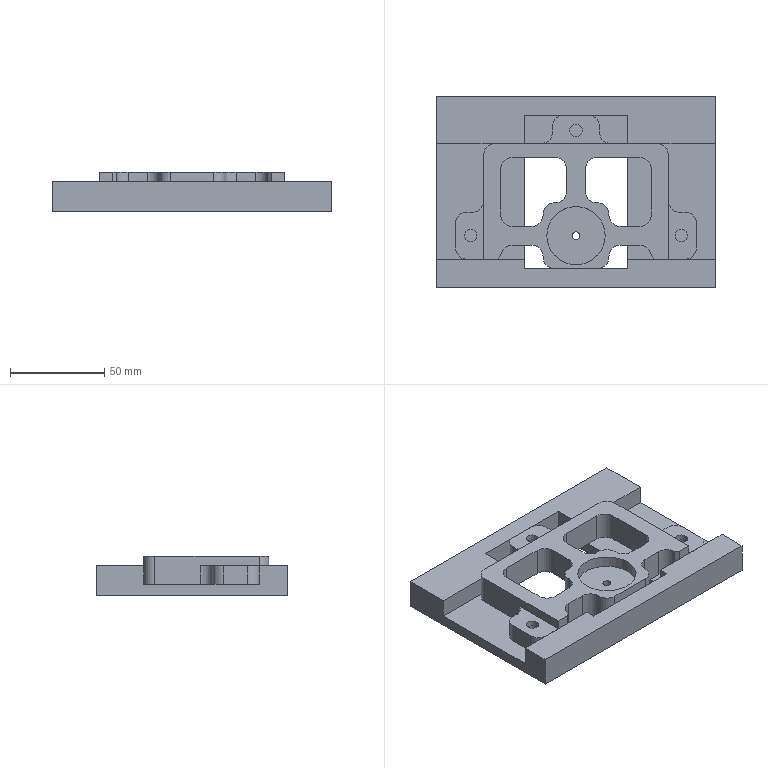NC program | NX | posted with a generic post | part box 148 x 101.5 x 21 mm
Whole program, first 1776 of 1973 lines:
N10 G17 G21 G94 G90
(FLOOR_WALL_COPY_1 , TOOL : D10)
N12 T04 M6
N14 G54
N16 G17 G0 G90 X72. Y-40.747 S9505 M3
N18 G43 Z30. H4
N20 Z6.025
N22 G94 G1 Z3.025 F2500.
N24 X69.
N26 X-69.
N28 Y-35.903
N30 X69.
N32 Y-31.06
N34 X-69.
N36 Y-26.216
N38 X69.
N40 Y-21.373
N42 X-69.
N44 Y-16.529
N46 X69.
N48 Y-11.686
N50 X-69.
N52 Y-6.842
N54 X69.
N56 Y-1.999
N58 X-69.
N60 Y2.845
N62 X69.
N64 Y7.689
N66 X-69.
N68 Y12.532
N70 X69.
N72 Y17.376
N74 X-69.
N76 Y22.219
N78 X69.
N80 Y27.063
N82 X-69.
N84 Y31.906
N86 X69.
N88 Y36.75
N90 X-69.
N92 X-72.
N94 Z6.025
N96 G0 Z30.
N98 X72. Y-40.747
N100 Z5.05
N102 G1 Z2.05
N104 X69.
N106 X-69.
N108 Y-35.903
N110 X69.
N112 Y-31.06
N114 X-69.
N116 Y-26.216
N118 X69.
N120 Y-21.373
N122 X-69.
N124 Y-16.529
N126 X69.
N128 Y-11.686
N130 X-69.
N132 Y-6.842
N134 X69.
N136 Y-1.999
N138 X-69.
N140 Y2.845
N142 X69.
N144 Y7.689
N146 X-69.
N148 Y12.532
N150 X69.
N152 Y17.376
N154 X-69.
N156 Y22.219
N158 X69.
N160 Y27.063
N162 X-69.
N164 Y31.906
N166 X69.
N168 Y36.75
N170 X-69.
N172 X-72.
N174 Z5.05
N176 G0 Z30.
N178 X72. Y-40.747
N180 Z4.075
N182 G1 Z1.075
N184 X69.
N186 X-69.
N188 Y-35.903
N190 X69.
N192 Y-31.06
N194 X-69.
N196 Y-26.216
N198 X69.
N200 Y-21.373
N202 X-69.
N204 Y-16.529
N206 X69.
N208 Y-11.686
N210 X-69.
N212 Y-6.842
N214 X69.
N216 Y-1.999
N218 X-69.
N220 Y2.845
N222 X69.
N224 Y7.689
N226 X-69.
N228 Y12.532
N230 X69.
N232 Y17.376
N234 X-69.
N236 Y22.219
N238 X69.
N240 Y27.063
N242 X-69.
N244 Y31.906
N246 X69.
N248 Y36.75
N250 X-69.
N252 X-72.
N254 Z4.075
N256 G0 Z30.
N258 X72. Y-40.747
N260 Z3.1
N262 G1 Z0.1
N264 X69.
N266 X-69.
N268 Y-35.903
N270 X69.
N272 Y-31.06
N274 X-69.
N276 Y-26.216
N278 X69.
N280 Y-21.373
N282 X-69.
N284 Y-16.529
N286 X69.
N288 Y-11.686
N290 X-69.
N292 Y-6.842
N294 X69.
N296 Y-1.999
N298 X-69.
N300 Y2.845
N302 X69.
N304 Y7.689
N306 X-69.
N308 Y12.532
N310 X69.
N312 Y17.376
N314 X-69.
N316 Y22.219
N318 X69.
N320 Y27.063
N322 X-69.
N324 Y31.906
N326 X69.
N328 Y36.75
N330 X-69.
N332 X-72.
N334 Z3.1
N336 G0 Z30.
(FLOOR_WALL_COPY_1_COPY , TOOL : D10)
N338 X21.949 Y-33.897
N340 Z3.021
N342 G1 Z0.021 F2200.
N344 X17.776 Y-31.299
N346 G3 X17.647 Y-31.75 R0.853
N348 G1 Y-34.75
N350 G2 X6.5 Y-45.897 R11.147
N352 G1 X-6.5
N354 G2 X-17.647 Y-34.75 R11.147
N356 G1 Y-31.75
N358 G3 X-18.5 Y-30.897 R0.853
N360 G1 X-43.
N362 G2 X-54.147 Y-19.75 R11.147
N364 G1 Y4.75
N366 G3 X-55. Y5.603 R0.853
N368 G1 X-58.
N370 G2 X-69.147 Y16.75 R11.147
N372 G1 Y29.75
N374 G2 X-58. Y40.897 R11.147
N376 G1 X-39.946
N378 X-34.979 Y36.231
N380 X-34.851 Y34.197
N382 G3 X-34. Y33.397 R0.853
N384 G1 X-23.5
N386 G3 X-22.679 Y34.019 R0.853
N388 G1 X-22.65 Y34.011
N390 Y11.75
N392 G3 X-11.5 Y0.6 R11.15
N394 G1 X11.5
N396 G3 X22.65 Y11.75 R11.15
N398 G1 Y34.011
N400 X22.679 Y34.019
N402 G3 X23.5 Y33.397 R0.853
N404 G1 X34.
N406 G3 X34.855 Y34.255 R0.855
N408 G1 X34.979 Y36.231
N410 X39.946 Y40.897
N412 X58.
N414 G2 X69.147 Y29.75 R11.147
N416 G1 Y16.75
N418 G2 X58. Y5.603 R11.147
N420 G1 X55.
N422 G3 X54.147 Y4.75 R0.853
N424 G1 Y-19.75
N426 G2 X43. Y-30.897 R11.147
N428 G1 X18.5
N430 G3 X17.776 Y-31.299 R0.853
N432 G1 X13.531 Y-28.657
N434 G3 X12.647 Y-31.75 R5.853
N436 G1 Y-34.75
N438 G2 X6.5 Y-40.897 R6.147
N440 G1 X-6.5
N442 G2 X-12.647 Y-34.75 R6.147
N444 G1 Y-31.75
N446 G3 X-18.5 Y-25.897 R5.853
N448 G1 X-43.
N450 G2 X-49.147 Y-19.75 R6.147
N452 G1 Y4.75
N454 G3 X-55. Y10.603 R5.853
N456 G1 X-58.
N458 G2 X-64.147 Y16.75 R6.147
N460 G1 Y29.75
N462 G2 X-58. Y35.897 R6.147
N464 G1 X-41.926
N466 X-39.845 Y33.942
N468 G3 X-34. Y28.397 R5.853
N470 G1 X-27.65
N472 Y11.75
N474 G3 X-11.5 Y-4.4 R16.15
N476 G1 X11.5
N478 G3 X27.65 Y11.75 R16.15
N480 G1 Y28.397
N482 X34.002
N484 G3 X39.567 Y32.442 R5.853
N486 X39.845 Y33.942 R5.853
N488 G1 X41.926 Y35.897
N490 X58.
N492 G2 X64.147 Y29.75 R6.147
N494 G1 Y16.75
N496 G2 X58. Y10.603 R6.147
N498 G1 X55.
N500 G3 X49.147 Y4.75 R5.853
N502 G1 Y-19.75
N504 G2 X43. Y-25.897 R6.147
N506 G1 X18.5
N508 G3 X13.531 Y-28.657 R5.853
N510 G1 X9.286 Y-26.015
N512 G3 X7.647 Y-31.75 R10.853
N514 G1 Y-34.75
N516 G2 X6.5 Y-35.897 R1.147
N518 G1 X-6.5
N520 G2 X-7.647 Y-34.75 R1.147
N522 G1 Y-31.75
N524 G3 X-18.5 Y-20.897 R10.853
N526 G1 X-43.
N528 G2 X-44.147 Y-19.75 R1.147
N530 G1 Y4.75
N532 G3 X-55. Y15.603 R10.853
N534 G1 X-58.
N536 G2 X-59.147 Y16.75 R1.147
N538 G1 Y29.75
N540 G2 X-58. Y30.897 R1.147
N542 G1 X-44.322
N544 G3 X-34. Y23.397 R10.853
N546 G1 X-32.65
N548 Y11.75
N550 G3 X-11.5 Y-9.4 R21.15
N552 G1 X11.5
N554 G3 X32.65 Y11.75 R21.15
N556 G1 Y23.397
N558 X34.004
N560 G3 X44.322 Y30.897 R10.853
N562 G1 X58.
N564 G2 X59.147 Y29.75 R1.147
N566 G1 Y16.75
N568 G2 X58. Y15.603 R1.147
N570 G1 X55.
N572 G3 X44.147 Y4.75 R10.853
N574 G1 Y-19.75
N576 G2 X43. Y-20.897 R1.147
N578 G1 X18.5
N580 G3 X9.286 Y-26.015 R10.853
N582 G1 X5.041 Y-23.373
N584 G3 X2.67 Y-30.897 R15.853
N586 G1 X-2.67
N588 G3 X-18.5 Y-15.897 R15.853
N590 G1 X-39.147
N592 Y4.75
N594 G3 X-54.147 Y20.58 R15.853
N596 G1 Y25.897
N598 X-47.474
N600 G3 X-37.65 Y18.823 R15.853
N602 G1 Y11.75
N604 G3 X-29.455 Y-7.262 R26.15
N606 G1 X-32.888 Y-10.897
N608 X-34.147
N610 Y-9.638
N612 G3 X-32.888 Y-10.897 R31.15
N614 G1 X-29.455 Y-7.262
N616 G3 X-11.5 Y-14.4 R26.15
N618 G1 X11.5
N620 G3 X37.65 Y11.75 R26.15
N622 G1 Y18.823
N624 G3 X47.474 Y25.897 R15.853
N626 G1 X54.147
N628 Y20.58
N630 G3 X39.147 Y4.75 R15.853
N632 G1 Y-15.897
N634 X32.888
N636 Y-10.897
N638 G3 X34.147 Y-9.638 R31.15
N640 G1 Y-10.897
N642 X32.888
N644 Y-15.897
N646 X18.5
N648 G3 X5.041 Y-23.373 R15.853
N650 G1 X0.796 Y-20.731
N652 G3 X0. Y-22.127 R20.853
N654 X-1.697 Y-19.4 R20.853
N656 G1 X1.697
N658 G3 X0.796 Y-20.731 R20.853
N660 G1 X3.343 Y-22.316
N662 Z3.021
N664 G0 Z30.
N666 X21.949 Y-33.897
N668 Z2.043
N670 G1 Z-0.957
N672 X17.776 Y-31.299
N674 G3 X17.647 Y-31.75 R0.853
N676 G1 Y-34.75
N678 G2 X6.5 Y-45.897 R11.147
N680 G1 X-6.5
N682 G2 X-17.647 Y-34.75 R11.147
N684 G1 Y-31.75
N686 G3 X-18.5 Y-30.897 R0.853
N688 G1 X-43.
N690 G2 X-54.147 Y-19.75 R11.147
N692 G1 Y4.75
N694 G3 X-55. Y5.603 R0.853
N696 G1 X-58.
N698 G2 X-69.147 Y16.75 R11.147
N700 G1 Y29.75
N702 G2 X-58. Y40.897 R11.147
N704 G1 X-39.946
N706 X-34.979 Y36.231
N708 X-34.851 Y34.197
N710 G3 X-34. Y33.397 R0.853
N712 G1 X-23.5
N714 G3 X-22.679 Y34.019 R0.853
N716 G1 X-22.65 Y34.011
N718 Y11.75
N720 G3 X-11.5 Y0.6 R11.15
N722 G1 X11.5
N724 G3 X22.65 Y11.75 R11.15
N726 G1 Y34.011
N728 X22.679 Y34.019
N730 G3 X23.5 Y33.397 R0.853
N732 G1 X34.
N734 G3 X34.855 Y34.255 R0.855
N736 G1 X34.979 Y36.231
N738 X39.946 Y40.897
N740 X58.
N742 G2 X69.147 Y29.75 R11.147
N744 G1 Y16.75
N746 G2 X58. Y5.603 R11.147
N748 G1 X55.
N750 G3 X54.147 Y4.75 R0.853
N752 G1 Y-19.75
N754 G2 X43. Y-30.897 R11.147
N756 G1 X18.5
N758 G3 X17.776 Y-31.299 R0.853
N760 G1 X13.531 Y-28.657
N762 G3 X12.647 Y-31.75 R5.853
N764 G1 Y-34.75
N766 G2 X6.5 Y-40.897 R6.147
N768 G1 X-6.5
N770 G2 X-12.647 Y-34.75 R6.147
N772 G1 Y-31.75
N774 G3 X-18.5 Y-25.897 R5.853
N776 G1 X-43.
N778 G2 X-49.147 Y-19.75 R6.147
N780 G1 Y4.75
N782 G3 X-55. Y10.603 R5.853
N784 G1 X-58.
N786 G2 X-64.147 Y16.75 R6.147
N788 G1 Y29.75
N790 G2 X-58. Y35.897 R6.147
N792 G1 X-41.926
N794 X-39.845 Y33.942
N796 G3 X-34. Y28.397 R5.853
N798 G1 X-27.65
N800 Y11.75
N802 G3 X-11.5 Y-4.4 R16.15
N804 G1 X11.5
N806 G3 X27.65 Y11.75 R16.15
N808 G1 Y28.397
N810 X34.002
N812 G3 X39.567 Y32.442 R5.853
N814 X39.845 Y33.942 R5.853
N816 G1 X41.926 Y35.897
N818 X58.
N820 G2 X64.147 Y29.75 R6.147
N822 G1 Y16.75
N824 G2 X58. Y10.603 R6.147
N826 G1 X55.
N828 G3 X49.147 Y4.75 R5.853
N830 G1 Y-19.75
N832 G2 X43. Y-25.897 R6.147
N834 G1 X18.5
N836 G3 X13.531 Y-28.657 R5.853
N838 G1 X9.286 Y-26.015
N840 G3 X7.647 Y-31.75 R10.853
N842 G1 Y-34.75
N844 G2 X6.5 Y-35.897 R1.147
N846 G1 X-6.5
N848 G2 X-7.647 Y-34.75 R1.147
N850 G1 Y-31.75
N852 G3 X-18.5 Y-20.897 R10.853
N854 G1 X-43.
N856 G2 X-44.147 Y-19.75 R1.147
N858 G1 Y4.75
N860 G3 X-55. Y15.603 R10.853
N862 G1 X-58.
N864 G2 X-59.147 Y16.75 R1.147
N866 G1 Y29.75
N868 G2 X-58. Y30.897 R1.147
N870 G1 X-44.322
N872 G3 X-34. Y23.397 R10.853
N874 G1 X-32.65
N876 Y11.75
N878 G3 X-11.5 Y-9.4 R21.15
N880 G1 X11.5
N882 G3 X32.65 Y11.75 R21.15
N884 G1 Y23.397
N886 X34.004
N888 G3 X44.322 Y30.897 R10.853
N890 G1 X58.
N892 G2 X59.147 Y29.75 R1.147
N894 G1 Y16.75
N896 G2 X58. Y15.603 R1.147
N898 G1 X55.
N900 G3 X44.147 Y4.75 R10.853
N902 G1 Y-19.75
N904 G2 X43. Y-20.897 R1.147
N906 G1 X18.5
N908 G3 X9.286 Y-26.015 R10.853
N910 G1 X5.041 Y-23.373
N912 G3 X2.67 Y-30.897 R15.853
N914 G1 X-2.67
N916 G3 X-18.5 Y-15.897 R15.853
N918 G1 X-39.147
N920 Y4.75
N922 G3 X-54.147 Y20.58 R15.853
N924 G1 Y25.897
N926 X-47.474
N928 G3 X-37.65 Y18.823 R15.853
N930 G1 Y11.75
N932 G3 X-29.455 Y-7.262 R26.15
N934 G1 X-32.888 Y-10.897
N936 X-34.147
N938 Y-9.638
N940 G3 X-32.888 Y-10.897 R31.15
N942 G1 X-29.455 Y-7.262
N944 G3 X-11.5 Y-14.4 R26.15
N946 G1 X11.5
N948 G3 X37.65 Y11.75 R26.15
N950 G1 Y18.823
N952 G3 X47.474 Y25.897 R15.853
N954 G1 X54.147
N956 Y20.58
N958 G3 X39.147 Y4.75 R15.853
N960 G1 Y-15.897
N962 X32.888
N964 Y-10.897
N966 G3 X34.147 Y-9.638 R31.15
N968 G1 Y-10.897
N970 X32.888
N972 Y-15.897
N974 X18.5
N976 G3 X5.041 Y-23.373 R15.853
N978 G1 X0.796 Y-20.731
N980 G3 X0. Y-22.127 R20.853
N982 X-1.697 Y-19.4 R20.853
N984 G1 X1.697
N986 G3 X0.796 Y-20.731 R20.853
N988 G1 X3.343 Y-22.316
N990 Z2.043
N992 G0 Z30.
N994 X21.949 Y-33.897
N996 Z1.064
N998 G1 Z-1.936
N1000 X17.776 Y-31.299
N1002 G3 X17.647 Y-31.75 R0.853
N1004 G1 Y-34.75
N1006 G2 X6.5 Y-45.897 R11.147
N1008 G1 X-6.5
N1010 G2 X-17.647 Y-34.75 R11.147
N1012 G1 Y-31.75
N1014 G3 X-18.5 Y-30.897 R0.853
N1016 G1 X-43.
N1018 G2 X-54.147 Y-19.75 R11.147
N1020 G1 Y4.75
N1022 G3 X-55. Y5.603 R0.853
N1024 G1 X-58.
N1026 G2 X-69.147 Y16.75 R11.147
N1028 G1 Y29.75
N1030 G2 X-58. Y40.897 R11.147
N1032 G1 X-39.946
N1034 X-34.979 Y36.231
N1036 X-34.851 Y34.197
N1038 G3 X-34. Y33.397 R0.853
N1040 G1 X-23.5
N1042 G3 X-22.679 Y34.019 R0.853
N1044 G1 X-22.65 Y34.011
N1046 Y11.75
N1048 G3 X-11.5 Y0.6 R11.15
N1050 G1 X11.5
N1052 G3 X22.65 Y11.75 R11.15
N1054 G1 Y34.011
N1056 X22.679 Y34.019
N1058 G3 X23.5 Y33.397 R0.853
N1060 G1 X34.
N1062 G3 X34.855 Y34.255 R0.855
N1064 G1 X34.979 Y36.231
N1066 X39.946 Y40.897
N1068 X58.
N1070 G2 X69.147 Y29.75 R11.147
N1072 G1 Y16.75
N1074 G2 X58. Y5.603 R11.147
N1076 G1 X55.
N1078 G3 X54.147 Y4.75 R0.853
N1080 G1 Y-19.75
N1082 G2 X43. Y-30.897 R11.147
N1084 G1 X18.5
N1086 G3 X17.776 Y-31.299 R0.853
N1088 G1 X13.531 Y-28.657
N1090 G3 X12.647 Y-31.75 R5.853
N1092 G1 Y-34.75
N1094 G2 X6.5 Y-40.897 R6.147
N1096 G1 X-6.5
N1098 G2 X-12.647 Y-34.75 R6.147
N1100 G1 Y-31.75
N1102 G3 X-18.5 Y-25.897 R5.853
N1104 G1 X-43.
N1106 G2 X-49.147 Y-19.75 R6.147
N1108 G1 Y4.75
N1110 G3 X-55. Y10.603 R5.853
N1112 G1 X-58.
N1114 G2 X-64.147 Y16.75 R6.147
N1116 G1 Y29.75
N1118 G2 X-58. Y35.897 R6.147
N1120 G1 X-41.926
N1122 X-39.845 Y33.942
N1124 G3 X-34. Y28.397 R5.853
N1126 G1 X-27.65
N1128 Y11.75
N1130 G3 X-11.5 Y-4.4 R16.15
N1132 G1 X11.5
N1134 G3 X27.65 Y11.75 R16.15
N1136 G1 Y28.397
N1138 X34.002
N1140 G3 X39.567 Y32.442 R5.853
N1142 X39.845 Y33.942 R5.853
N1144 G1 X41.926 Y35.897
N1146 X58.
N1148 G2 X64.147 Y29.75 R6.147
N1150 G1 Y16.75
N1152 G2 X58. Y10.603 R6.147
N1154 G1 X55.
N1156 G3 X49.147 Y4.75 R5.853
N1158 G1 Y-19.75
N1160 G2 X43. Y-25.897 R6.147
N1162 G1 X18.5
N1164 G3 X13.531 Y-28.657 R5.853
N1166 G1 X9.286 Y-26.015
N1168 G3 X7.647 Y-31.75 R10.853
N1170 G1 Y-34.75
N1172 G2 X6.5 Y-35.897 R1.147
N1174 G1 X-6.5
N1176 G2 X-7.647 Y-34.75 R1.147
N1178 G1 Y-31.75
N1180 G3 X-18.5 Y-20.897 R10.853
N1182 G1 X-43.
N1184 G2 X-44.147 Y-19.75 R1.147
N1186 G1 Y4.75
N1188 G3 X-55. Y15.603 R10.853
N1190 G1 X-58.
N1192 G2 X-59.147 Y16.75 R1.147
N1194 G1 Y29.75
N1196 G2 X-58. Y30.897 R1.147
N1198 G1 X-44.322
N1200 G3 X-34. Y23.397 R10.853
N1202 G1 X-32.65
N1204 Y11.75
N1206 G3 X-11.5 Y-9.4 R21.15
N1208 G1 X11.5
N1210 G3 X32.65 Y11.75 R21.15
N1212 G1 Y23.397
N1214 X34.004
N1216 G3 X44.322 Y30.897 R10.853
N1218 G1 X58.
N1220 G2 X59.147 Y29.75 R1.147
N1222 G1 Y16.75
N1224 G2 X58. Y15.603 R1.147
N1226 G1 X55.
N1228 G3 X44.147 Y4.75 R10.853
N1230 G1 Y-19.75
N1232 G2 X43. Y-20.897 R1.147
N1234 G1 X18.5
N1236 G3 X9.286 Y-26.015 R10.853
N1238 G1 X5.041 Y-23.373
N1240 G3 X2.67 Y-30.897 R15.853
N1242 G1 X-2.67
N1244 G3 X-18.5 Y-15.897 R15.853
N1246 G1 X-39.147
N1248 Y4.75
N1250 G3 X-54.147 Y20.58 R15.853
N1252 G1 Y25.897
N1254 X-47.474
N1256 G3 X-37.65 Y18.823 R15.853
N1258 G1 Y11.75
N1260 G3 X-29.455 Y-7.262 R26.15
N1262 G1 X-32.888 Y-10.897
N1264 X-34.147
N1266 Y-9.638
N1268 G3 X-32.888 Y-10.897 R31.15
N1270 G1 X-29.455 Y-7.262
N1272 G3 X-11.5 Y-14.4 R26.15
N1274 G1 X11.5
N1276 G3 X37.65 Y11.75 R26.15
N1278 G1 Y18.823
N1280 G3 X47.474 Y25.897 R15.853
N1282 G1 X54.147
N1284 Y20.58
N1286 G3 X39.147 Y4.75 R15.853
N1288 G1 Y-15.897
N1290 X32.888
N1292 Y-10.897
N1294 G3 X34.147 Y-9.638 R31.15
N1296 G1 Y-10.897
N1298 X32.888
N1300 Y-15.897
N1302 X18.5
N1304 G3 X5.041 Y-23.373 R15.853
N1306 G1 X0.796 Y-20.731
N1308 G3 X0. Y-22.127 R20.853
N1310 X-1.697 Y-19.4 R20.853
N1312 G1 X1.697
N1314 G3 X0.796 Y-20.731 R20.853
N1316 G1 X3.343 Y-22.316
N1318 Z1.064
N1320 G0 Z30.
N1322 X21.949 Y-33.897
N1324 Z0.086
N1326 G1 Z-2.914
N1328 X17.776 Y-31.299
N1330 G3 X17.647 Y-31.75 R0.853
N1332 G1 Y-34.75
N1334 G2 X6.5 Y-45.897 R11.147
N1336 G1 X-6.5
N1338 G2 X-17.647 Y-34.75 R11.147
N1340 G1 Y-31.75
N1342 G3 X-18.5 Y-30.897 R0.853
N1344 G1 X-43.
N1346 G2 X-54.147 Y-19.75 R11.147
N1348 G1 Y4.75
N1350 G3 X-55. Y5.603 R0.853
N1352 G1 X-58.
N1354 G2 X-69.147 Y16.75 R11.147
N1356 G1 Y29.75
N1358 G2 X-58. Y40.897 R11.147
N1360 G1 X-39.946
N1362 X-34.979 Y36.231
N1364 X-34.851 Y34.197
N1366 G3 X-34. Y33.397 R0.853
N1368 G1 X-23.5
N1370 G3 X-22.679 Y34.019 R0.853
N1372 G1 X-22.65 Y34.011
N1374 Y11.75
N1376 G3 X-11.5 Y0.6 R11.15
N1378 G1 X11.5
N1380 G3 X22.65 Y11.75 R11.15
N1382 G1 Y34.011
N1384 X22.679 Y34.019
N1386 G3 X23.5 Y33.397 R0.853
N1388 G1 X34.
N1390 G3 X34.855 Y34.255 R0.855
N1392 G1 X34.979 Y36.231
N1394 X39.946 Y40.897
N1396 X58.
N1398 G2 X69.147 Y29.75 R11.147
N1400 G1 Y16.75
N1402 G2 X58. Y5.603 R11.147
N1404 G1 X55.
N1406 G3 X54.147 Y4.75 R0.853
N1408 G1 Y-19.75
N1410 G2 X43. Y-30.897 R11.147
N1412 G1 X18.5
N1414 G3 X17.776 Y-31.299 R0.853
N1416 G1 X13.531 Y-28.657
N1418 G3 X12.647 Y-31.75 R5.853
N1420 G1 Y-34.75
N1422 G2 X6.5 Y-40.897 R6.147
N1424 G1 X-6.5
N1426 G2 X-12.647 Y-34.75 R6.147
N1428 G1 Y-31.75
N1430 G3 X-18.5 Y-25.897 R5.853
N1432 G1 X-43.
N1434 G2 X-49.147 Y-19.75 R6.147
N1436 G1 Y4.75
N1438 G3 X-55. Y10.603 R5.853
N1440 G1 X-58.
N1442 G2 X-64.147 Y16.75 R6.147
N1444 G1 Y29.75
N1446 G2 X-58. Y35.897 R6.147
N1448 G1 X-41.926
N1450 X-39.845 Y33.942
N1452 G3 X-34. Y28.397 R5.853
N1454 G1 X-27.65
N1456 Y11.75
N1458 G3 X-11.5 Y-4.4 R16.15
N1460 G1 X11.5
N1462 G3 X27.65 Y11.75 R16.15
N1464 G1 Y28.397
N1466 X34.002
N1468 G3 X39.567 Y32.442 R5.853
N1470 X39.845 Y33.942 R5.853
N1472 G1 X41.926 Y35.897
N1474 X58.
N1476 G2 X64.147 Y29.75 R6.147
N1478 G1 Y16.75
N1480 G2 X58. Y10.603 R6.147
N1482 G1 X55.
N1484 G3 X49.147 Y4.75 R5.853
N1486 G1 Y-19.75
N1488 G2 X43. Y-25.897 R6.147
N1490 G1 X18.5
N1492 G3 X13.531 Y-28.657 R5.853
N1494 G1 X9.286 Y-26.015
N1496 G3 X7.647 Y-31.75 R10.853
N1498 G1 Y-34.75
N1500 G2 X6.5 Y-35.897 R1.147
N1502 G1 X-6.5
N1504 G2 X-7.647 Y-34.75 R1.147
N1506 G1 Y-31.75
N1508 G3 X-18.5 Y-20.897 R10.853
N1510 G1 X-43.
N1512 G2 X-44.147 Y-19.75 R1.147
N1514 G1 Y4.75
N1516 G3 X-55. Y15.603 R10.853
N1518 G1 X-58.
N1520 G2 X-59.147 Y16.75 R1.147
N1522 G1 Y29.75
N1524 G2 X-58. Y30.897 R1.147
N1526 G1 X-44.322
N1528 G3 X-34. Y23.397 R10.853
N1530 G1 X-32.65
N1532 Y11.75
N1534 G3 X-11.5 Y-9.4 R21.15
N1536 G1 X11.5
N1538 G3 X32.65 Y11.75 R21.15
N1540 G1 Y23.397
N1542 X34.004
N1544 G3 X44.322 Y30.897 R10.853
N1546 G1 X58.
N1548 G2 X59.147 Y29.75 R1.147
N1550 G1 Y16.75
N1552 G2 X58. Y15.603 R1.147
N1554 G1 X55.
N1556 G3 X44.147 Y4.75 R10.853
N1558 G1 Y-19.75
N1560 G2 X43. Y-20.897 R1.147
N1562 G1 X18.5
N1564 G3 X9.286 Y-26.015 R10.853
N1566 G1 X5.041 Y-23.373
N1568 G3 X2.67 Y-30.897 R15.853
N1570 G1 X-2.67
N1572 G3 X-18.5 Y-15.897 R15.853
N1574 G1 X-39.147
N1576 Y4.75
N1578 G3 X-54.147 Y20.58 R15.853
N1580 G1 Y25.897
N1582 X-47.474
N1584 G3 X-37.65 Y18.823 R15.853
N1586 G1 Y11.75
N1588 G3 X-29.455 Y-7.262 R26.15
N1590 G1 X-32.888 Y-10.897
N1592 X-34.147
N1594 Y-9.638
N1596 G3 X-32.888 Y-10.897 R31.15
N1598 G1 X-29.455 Y-7.262
N1600 G3 X-11.5 Y-14.4 R26.15
N1602 G1 X11.5
N1604 G3 X37.65 Y11.75 R26.15
N1606 G1 Y18.823
N1608 G3 X47.474 Y25.897 R15.853
N1610 G1 X54.147
N1612 Y20.58
N1614 G3 X39.147 Y4.75 R15.853
N1616 G1 Y-15.897
N1618 X32.888
N1620 Y-10.897
N1622 G3 X34.147 Y-9.638 R31.15
N1624 G1 Y-10.897
N1626 X32.888
N1628 Y-15.897
N1630 X18.5
N1632 G3 X5.041 Y-23.373 R15.853
N1634 G1 X0.796 Y-20.731
N1636 G3 X0. Y-22.127 R20.853
N1638 X-1.697 Y-19.4 R20.853
N1640 G1 X1.697
N1642 G3 X0.796 Y-20.731 R20.853
N1644 G1 X3.343 Y-22.316
N1646 Z0.086
N1648 G0 Z30.
N1650 X21.949 Y-33.897
N1652 Z-0.893
N1654 G1 Z-3.893
N1656 X17.776 Y-31.299
N1658 G3 X17.647 Y-31.75 R0.853
N1660 G1 Y-34.75
N1662 G2 X6.5 Y-45.897 R11.147
N1664 G1 X-6.5
N1666 G2 X-17.647 Y-34.75 R11.147
N1668 G1 Y-31.75
N1670 G3 X-18.5 Y-30.897 R0.853
N1672 G1 X-43.
N1674 G2 X-54.147 Y-19.75 R11.147
N1676 G1 Y4.75
N1678 G3 X-55. Y5.603 R0.853
N1680 G1 X-58.
N1682 G2 X-69.147 Y16.75 R11.147
N1684 G1 Y29.75
N1686 G2 X-58. Y40.897 R11.147
N1688 G1 X-39.946
N1690 X-34.979 Y36.231
N1692 X-34.851 Y34.197
N1694 G3 X-34. Y33.397 R0.853
N1696 G1 X-23.5
N1698 G3 X-22.679 Y34.019 R0.853
N1700 G1 X-22.65 Y34.011
N1702 Y11.75
N1704 G3 X-11.5 Y0.6 R11.15
N1706 G1 X11.5
N1708 G3 X22.65 Y11.75 R11.15
N1710 G1 Y34.011
N1712 X22.679 Y34.019
N1714 G3 X23.5 Y33.397 R0.853
N1716 G1 X34.
N1718 G3 X34.855 Y34.255 R0.855
N1720 G1 X34.979 Y36.231
N1722 X39.946 Y40.897
N1724 X58.
N1726 G2 X69.147 Y29.75 R11.147
N1728 G1 Y16.75
N1730 G2 X58. Y5.603 R11.147
N1732 G1 X55.
N1734 G3 X54.147 Y4.75 R0.853
N1736 G1 Y-19.75
N1738 G2 X43. Y-30.897 R11.147
N1740 G1 X18.5
N1742 G3 X17.776 Y-31.299 R0.853
N1744 G1 X13.531 Y-28.657
N1746 G3 X12.647 Y-31.75 R5.853
N1748 G1 Y-34.75
N1750 G2 X6.5 Y-40.897 R6.147
N1752 G1 X-6.5
N1754 G2 X-12.647 Y-34.75 R6.147
N1756 G1 Y-31.75
N1758 G3 X-18.5 Y-25.897 R5.853
N1760 G1 X-43.
N1762 G2 X-49.147 Y-19.75 R6.147
N1764 G1 Y4.75
N1766 G3 X-55. Y10.603 R5.853
N1768 G1 X-58.
N1770 G2 X-64.147 Y16.75 R6.147
N1772 G1 Y29.75
N1774 G2 X-58. Y35.897 R6.147
N1776 G1 X-41.926
N1778 X-39.845 Y33.942
N1780 G3 X-34. Y28.397 R5.853
N1782 G1 X-27.65
N1784 Y11.75
N1786 G3 X-11.5 Y-4.4 R16.15
N1788 G1 X11.5
N1790 G3 X27.65 Y11.75 R16.15
N1792 G1 Y28.397
N1794 X34.002
N1796 G3 X39.567 Y32.442 R5.853
N1798 X39.845 Y33.942 R5.853
N1800 G1 X41.926 Y35.897
N1802 X58.
N1804 G2 X64.147 Y29.75 R6.147
N1806 G1 Y16.75
N1808 G2 X58. Y10.603 R6.147
N1810 G1 X55.
N1812 G3 X49.147 Y4.75 R5.853
N1814 G1 Y-19.75
N1816 G2 X43. Y-25.897 R6.147
N1818 G1 X18.5
N1820 G3 X13.531 Y-28.657 R5.853
N1822 G1 X9.286 Y-26.015
N1824 G3 X7.647 Y-31.75 R10.853
N1826 G1 Y-34.75
N1828 G2 X6.5 Y-35.897 R1.147
N1830 G1 X-6.5
N1832 G2 X-7.647 Y-34.75 R1.147
N1834 G1 Y-31.75
N1836 G3 X-18.5 Y-20.897 R10.853
N1838 G1 X-43.
N1840 G2 X-44.147 Y-19.75 R1.147
N1842 G1 Y4.75
N1844 G3 X-55. Y15.603 R10.853
N1846 G1 X-58.
N1848 G2 X-59.147 Y16.75 R1.147
N1850 G1 Y29.75
N1852 G2 X-58. Y30.897 R1.147
N1854 G1 X-44.322
N1856 G3 X-34. Y23.397 R10.853
N1858 G1 X-32.65
N1860 Y11.75
N1862 G3 X-11.5 Y-9.4 R21.15
N1864 G1 X11.5
N1866 G3 X32.65 Y11.75 R21.15
N1868 G1 Y23.397
N1870 X34.004
N1872 G3 X44.322 Y30.897 R10.853
N1874 G1 X58.
N1876 G2 X59.147 Y29.75 R1.147
N1878 G1 Y16.75
N1880 G2 X58. Y15.603 R1.147
N1882 G1 X55.
N1884 G3 X44.147 Y4.75 R10.853
N1886 G1 Y-19.75
N1888 G2 X43. Y-20.897 R1.147
N1890 G1 X18.5
N1892 G3 X9.286 Y-26.015 R10.853
N1894 G1 X5.041 Y-23.373
N1896 G3 X2.67 Y-30.897 R15.853
N1898 G1 X-2.67
N1900 G3 X-18.5 Y-15.897 R15.853
N1902 G1 X-39.147
N1904 Y4.75
N1906 G3 X-54.147 Y20.58 R15.853
N1908 G1 Y25.897
N1910 X-47.474
N1912 G3 X-37.65 Y18.823 R15.853
N1914 G1 Y11.75
N1916 G3 X-29.455 Y-7.262 R26.15
N1918 G1 X-32.888 Y-10.897
N1920 X-34.147
N1922 Y-9.638
N1924 G3 X-32.888 Y-10.897 R31.15
N1926 G1 X-29.455 Y-7.262
N1928 G3 X-11.5 Y-14.4 R26.15
N1930 G1 X11.5
N1932 G3 X37.65 Y11.75 R26.15
N1934 G1 Y18.823
N1936 G3 X47.474 Y25.897 R15.853
N1938 G1 X54.147
N1940 Y20.58
N1942 G3 X39.147 Y4.75 R15.853
N1944 G1 Y-15.897
N1946 X32.888
N1948 Y-10.897
N1950 G3 X34.147 Y-9.638 R31.15
N1952 G1 Y-10.897
N1954 X32.888
N1956 Y-15.897
N1958 X18.5
N1960 G3 X5.041 Y-23.373 R15.853
N1962 G1 X0.796 Y-20.731
N1964 G3 X0. Y-22.127 R20.853
N1966 X-1.697 Y-19.4 R20.853
N1968 G1 X1.697
N1970 G3 X0.796 Y-20.731 R20.853
N1972 G1 X3.343 Y-22.316
N1974 Z-0.893
N1976 G0 Z30.
N1978 X21.949 Y-33.897
N1980 Z-1.871
N1982 G1 Z-4.871
N1984 X17.776 Y-31.299
N1986 G3 X17.647 Y-31.75 R0.853
N1988 G1 Y-34.75
N1990 G2 X6.5 Y-45.897 R11.147
N1992 G1 X-6.5
N1994 G2 X-17.647 Y-34.75 R11.147
N1996 G1 Y-31.75
N1998 G3 X-18.5 Y-30.897 R0.853
N2000 G1 X-43.
N2002 G2 X-54.147 Y-19.75 R11.147
N2004 G1 Y4.75
N2006 G3 X-55. Y5.603 R0.853
N2008 G1 X-58.
N2010 G2 X-69.147 Y16.75 R11.147
N2012 G1 Y29.75
N2014 G2 X-58. Y40.897 R11.147
N2016 G1 X-39.946
N2018 X-34.979 Y36.231
N2020 X-34.851 Y34.197
N2022 G3 X-34. Y33.397 R0.853
N2024 G1 X-23.5
N2026 G3 X-22.679 Y34.019 R0.853
N2028 G1 X-22.65 Y34.011
N2030 Y11.75
N2032 G3 X-11.5 Y0.6 R11.15
N2034 G1 X11.5
N2036 G3 X22.65 Y11.75 R11.15
N2038 G1 Y34.011
N2040 X22.679 Y34.019
N2042 G3 X23.5 Y33.397 R0.853
N2044 G1 X34.
N2046 G3 X34.855 Y34.255 R0.855
N2048 G1 X34.979 Y36.231
N2050 X39.946 Y40.897
N2052 X58.
N2054 G2 X69.147 Y29.75 R11.147
N2056 G1 Y16.75
N2058 G2 X58. Y5.603 R11.147
N2060 G1 X55.
N2062 G3 X54.147 Y4.75 R0.853
N2064 G1 Y-19.75
N2066 G2 X43. Y-30.897 R11.147
N2068 G1 X18.5
N2070 G3 X17.776 Y-31.299 R0.853
N2072 G1 X13.531 Y-28.657
N2074 G3 X12.647 Y-31.75 R5.853
N2076 G1 Y-34.75
N2078 G2 X6.5 Y-40.897 R6.147
N2080 G1 X-6.5
N2082 G2 X-12.647 Y-34.75 R6.147
N2084 G1 Y-31.75
N2086 G3 X-18.5 Y-25.897 R5.853
N2088 G1 X-43.
N2090 G2 X-49.147 Y-19.75 R6.147
N2092 G1 Y4.75
N2094 G3 X-55. Y10.603 R5.853
N2096 G1 X-58.
N2098 G2 X-64.147 Y16.75 R6.147
N2100 G1 Y29.75
N2102 G2 X-58. Y35.897 R6.147
N2104 G1 X-41.926
N2106 X-39.845 Y33.942
N2108 G3 X-34. Y28.397 R5.853
N2110 G1 X-27.65
N2112 Y11.75
N2114 G3 X-11.5 Y-4.4 R16.15
N2116 G1 X11.5
N2118 G3 X27.65 Y11.75 R16.15
N2120 G1 Y28.397
N2122 X34.002
N2124 G3 X39.567 Y32.442 R5.853
N2126 X39.845 Y33.942 R5.853
N2128 G1 X41.926 Y35.897
N2130 X58.
N2132 G2 X64.147 Y29.75 R6.147
N2134 G1 Y16.75
N2136 G2 X58. Y10.603 R6.147
N2138 G1 X55.
N2140 G3 X49.147 Y4.75 R5.853
N2142 G1 Y-19.75
N2144 G2 X43. Y-25.897 R6.147
N2146 G1 X18.5
N2148 G3 X13.531 Y-28.657 R5.853
N2150 G1 X9.286 Y-26.015
N2152 G3 X7.647 Y-31.75 R10.853
N2154 G1 Y-34.75
N2156 G2 X6.5 Y-35.897 R1.147
N2158 G1 X-6.5
N2160 G2 X-7.647 Y-34.75 R1.147
N2162 G1 Y-31.75
N2164 G3 X-18.5 Y-20.897 R10.853
N2166 G1 X-43.
N2168 G2 X-44.147 Y-19.75 R1.147
N2170 G1 Y4.75
N2172 G3 X-55. Y15.603 R10.853
N2174 G1 X-58.
N2176 G2 X-59.147 Y16.75 R1.147
N2178 G1 Y29.75
N2180 G2 X-58. Y30.897 R1.147
N2182 G1 X-44.322
N2184 G3 X-34. Y23.397 R10.853
N2186 G1 X-32.65
N2188 Y11.75
N2190 G3 X-11.5 Y-9.4 R21.15
N2192 G1 X11.5
N2194 G3 X32.65 Y11.75 R21.15
N2196 G1 Y23.397
N2198 X34.004
N2200 G3 X44.322 Y30.897 R10.853
N2202 G1 X58.
N2204 G2 X59.147 Y29.75 R1.147
N2206 G1 Y16.75
N2208 G2 X58. Y15.603 R1.147
N2210 G1 X55.
N2212 G3 X44.147 Y4.75 R10.853
N2214 G1 Y-19.75
N2216 G2 X43. Y-20.897 R1.147
N2218 G1 X18.5
N2220 G3 X9.286 Y-26.015 R10.853
N2222 G1 X5.041 Y-23.373
N2224 G3 X2.67 Y-30.897 R15.853
N2226 G1 X-2.67
N2228 G3 X-18.5 Y-15.897 R15.853
N2230 G1 X-39.147
N2232 Y4.75
N2234 G3 X-54.147 Y20.58 R15.853
N2236 G1 Y25.897
N2238 X-47.474
N2240 G3 X-37.65 Y18.823 R15.853
N2242 G1 Y11.75
N2244 G3 X-29.455 Y-7.262 R26.15
N2246 G1 X-32.888 Y-10.897
N2248 X-34.147
N2250 Y-9.638
N2252 G3 X-32.888 Y-10.897 R31.15
N2254 G1 X-29.455 Y-7.262
N2256 G3 X-11.5 Y-14.4 R26.15
N2258 G1 X11.5
N2260 G3 X37.65 Y11.75 R26.15
N2262 G1 Y18.823
N2264 G3 X47.474 Y25.897 R15.853
N2266 G1 X54.147
N2268 Y20.58
N2270 G3 X39.147 Y4.75 R15.853
N2272 G1 Y-15.897
N2274 X32.888
N2276 Y-10.897
N2278 G3 X34.147 Y-9.638 R31.15
N2280 G1 Y-10.897
N2282 X32.888
N2284 Y-15.897
N2286 X18.5
N2288 G3 X5.041 Y-23.373 R15.853
N2290 G1 X0.796 Y-20.731
N2292 G3 X0. Y-22.127 R20.853
N2294 X-1.697 Y-19.4 R20.853
N2296 G1 X1.697
N2298 G3 X0.796 Y-20.731 R20.853
N2300 G1 X3.343 Y-22.316
N2302 Z-1.871
N2304 G0 Z30.
N2306 X21.949 Y-33.897
N2308 Z-2.85
N2310 G1 Z-5.85
N2312 X17.776 Y-31.299
N2314 G3 X17.647 Y-31.75 R0.853
N2316 G1 Y-34.75
N2318 G2 X6.5 Y-45.897 R11.147
N2320 G1 X-6.5
N2322 G2 X-17.647 Y-34.75 R11.147
N2324 G1 Y-31.75
N2326 G3 X-18.5 Y-30.897 R0.853
N2328 G1 X-43.
N2330 G2 X-54.147 Y-19.75 R11.147
N2332 G1 Y4.75
N2334 G3 X-55. Y5.603 R0.853
N2336 G1 X-58.
N2338 G2 X-69.147 Y16.75 R11.147
N2340 G1 Y29.75
N2342 G2 X-58. Y40.897 R11.147
N2344 G1 X-39.946
N2346 X-34.979 Y36.231
N2348 X-34.851 Y34.197
N2350 G3 X-34. Y33.397 R0.853
N2352 G1 X-23.5
N2354 G3 X-22.679 Y34.019 R0.853
N2356 G1 X-22.65 Y34.011
N2358 Y11.75
N2360 G3 X-11.5 Y0.6 R11.15
N2362 G1 X11.5
N2364 G3 X22.65 Y11.75 R11.15
N2366 G1 Y34.011
N2368 X22.679 Y34.019
N2370 G3 X23.5 Y33.397 R0.853
N2372 G1 X34.
N2374 G3 X34.855 Y34.255 R0.855
N2376 G1 X34.979 Y36.231
N2378 X39.946 Y40.897
N2380 X58.
N2382 G2 X69.147 Y29.75 R11.147
N2384 G1 Y16.75
N2386 G2 X58. Y5.603 R11.147
N2388 G1 X55.
N2390 G3 X54.147 Y4.75 R0.853
N2392 G1 Y-19.75
N2394 G2 X43. Y-30.897 R11.147
N2396 G1 X18.5
N2398 G3 X17.776 Y-31.299 R0.853
N2400 G1 X13.531 Y-28.657
N2402 G3 X12.647 Y-31.75 R5.853
N2404 G1 Y-34.75
N2406 G2 X6.5 Y-40.897 R6.147
N2408 G1 X-6.5
N2410 G2 X-12.647 Y-34.75 R6.147
N2412 G1 Y-31.75
N2414 G3 X-18.5 Y-25.897 R5.853
N2416 G1 X-43.
N2418 G2 X-49.147 Y-19.75 R6.147
N2420 G1 Y4.75
N2422 G3 X-55. Y10.603 R5.853
N2424 G1 X-58.
N2426 G2 X-64.147 Y16.75 R6.147
N2428 G1 Y29.75
N2430 G2 X-58. Y35.897 R6.147
N2432 G1 X-41.926
N2434 X-39.845 Y33.942
N2436 G3 X-34. Y28.397 R5.853
N2438 G1 X-27.65
N2440 Y11.75
N2442 G3 X-11.5 Y-4.4 R16.15
N2444 G1 X11.5
N2446 G3 X27.65 Y11.75 R16.15
N2448 G1 Y28.397
N2450 X34.002
N2452 G3 X39.567 Y32.442 R5.853
N2454 X39.845 Y33.942 R5.853
N2456 G1 X41.926 Y35.897
N2458 X58.
N2460 G2 X64.147 Y29.75 R6.147
N2462 G1 Y16.75
N2464 G2 X58. Y10.603 R6.147
N2466 G1 X55.
N2468 G3 X49.147 Y4.75 R5.853
N2470 G1 Y-19.75
N2472 G2 X43. Y-25.897 R6.147
N2474 G1 X18.5
N2476 G3 X13.531 Y-28.657 R5.853
N2478 G1 X9.286 Y-26.015
N2480 G3 X7.647 Y-31.75 R10.853
N2482 G1 Y-34.75
N2484 G2 X6.5 Y-35.897 R1.147
N2486 G1 X-6.5
N2488 G2 X-7.647 Y-34.75 R1.147
N2490 G1 Y-31.75
N2492 G3 X-18.5 Y-20.897 R10.853
N2494 G1 X-43.
N2496 G2 X-44.147 Y-19.75 R1.147
N2498 G1 Y4.75
N2500 G3 X-55. Y15.603 R10.853
N2502 G1 X-58.
N2504 G2 X-59.147 Y16.75 R1.147
N2506 G1 Y29.75
N2508 G2 X-58. Y30.897 R1.147
N2510 G1 X-44.322
N2512 G3 X-34. Y23.397 R10.853
N2514 G1 X-32.65
N2516 Y11.75
N2518 G3 X-11.5 Y-9.4 R21.15
N2520 G1 X11.5
N2522 G3 X32.65 Y11.75 R21.15
N2524 G1 Y23.397
N2526 X34.004
N2528 G3 X44.322 Y30.897 R10.853
N2530 G1 X58.
N2532 G2 X59.147 Y29.75 R1.147
N2534 G1 Y16.75
N2536 G2 X58. Y15.603 R1.147
N2538 G1 X55.
N2540 G3 X44.147 Y4.75 R10.853
N2542 G1 Y-19.75
N2544 G2 X43. Y-20.897 R1.147
N2546 G1 X18.5
N2548 G3 X9.286 Y-26.015 R10.853
N2550 G1 X5.041 Y-23.373
N2552 G3 X2.67 Y-30.897 R15.853
N2554 G1 X-2.67
N2556 G3 X-18.5 Y-15.897 R15.853
N2558 G1 X-39.147
N2560 Y4.75
N2562 G3 X-54.147 Y20.58 R15.853
N2564 G1 Y25.897
N2566 X-47.474
N2568 G3 X-37.65 Y18.823 R15.853
N2570 G1 Y11.75
N2572 G3 X-29.455 Y-7.262 R26.15
N2574 G1 X-32.888 Y-10.897
N2576 X-34.147
N2578 Y-9.638
N2580 G3 X-32.888 Y-10.897 R31.15
N2582 G1 X-29.455 Y-7.262
N2584 G3 X-11.5 Y-14.4 R26.15
N2586 G1 X11.5
N2588 G3 X37.65 Y11.75 R26.15
N2590 G1 Y18.823
N2592 G3 X47.474 Y25.897 R15.853
N2594 G1 X54.147
N2596 Y20.58
N2598 G3 X39.147 Y4.75 R15.853
N2600 G1 Y-15.897
N2602 X32.888
N2604 Y-10.897
N2606 G3 X34.147 Y-9.638 R31.15
N2608 G1 Y-10.897
N2610 X32.888
N2612 Y-15.897
N2614 X18.5
N2616 G3 X5.041 Y-23.373 R15.853
N2618 G1 X0.796 Y-20.731
N2620 G3 X0. Y-22.127 R20.853
N2622 X-1.697 Y-19.4 R20.853
N2624 G1 X1.697
N2626 G3 X0.796 Y-20.731 R20.853
N2628 G1 X3.343 Y-22.316
N2630 Z-2.85
N2632 G0 Z30.
(FLOOR_WALL_COPY_1_COPY_COPY , TOOL : D10)
N2634 X-10.097 Y24.604
N2636 Z4.
N2638 G1 X-9.834 Y26.068 Z3.601
N2640 X-9.066 Y27.989 Z3.047
N2642 X-7.928 Y29.715 Z2.493
N2644 X-6.465 Y31.178 Z1.939
N2646 X-4.739 Y32.316 Z1.385
N2648 X-2.818 Y33.084 Z0.831
N2650 X-0.783 Y33.45 Z0.276
N2652 X0. Z0.067
N2654 G2 X10.2 Y23.25 R10.2
N2656 X0. Y33.45 R-10.2
N2658 G1 Y28.45
N2660 G2 X5.2 Y23.25 R5.2
N2662 X0. Y28.45 R-5.2
N2664 G1 Y23.45
N2666 G2 X0.2 Y23.25 R0.2
N2668 X0. Y23.45 R-0.2
N2670 G1 Y26.45
N2672 Z3.067
N2674 G0 Z30.
N2676 X-10.097 Y24.604
N2678 Z3.067
N2680 G1 X-9.834 Y26.068 Z2.668
N2682 X-9.066 Y27.989 Z2.114
N2684 X-7.928 Y29.715 Z1.56
N2686 X-6.465 Y31.178 Z1.006
N2688 X-4.739 Y32.316 Z0.451
N2690 X-2.818 Y33.084 Z-0.103
N2692 X-0.783 Y33.45 Z-0.657
N2694 X0. Z-0.867
N2696 G2 X10.2 Y23.25 R10.2
N2698 X0. Y33.45 R-10.2
N2700 G1 Y28.45
N2702 G2 X5.2 Y23.25 R5.2
N2704 X0. Y28.45 R-5.2
N2706 G1 Y23.45
N2708 G2 X0.2 Y23.25 R0.2
N2710 X0. Y23.45 R-0.2
N2712 G1 Y26.45
N2714 Z2.133
N2716 G0 Z30.
N2718 X-10.097 Y24.604
N2720 Z2.133
N2722 G1 X-9.834 Y26.068 Z1.735
N2724 X-9.066 Y27.989 Z1.181
N2726 X-7.928 Y29.715 Z0.626
N2728 X-6.465 Y31.178 Z0.072
N2730 X-4.739 Y32.316 Z-0.482
N2732 X-2.818 Y33.084 Z-1.036
N2734 X-0.783 Y33.45 Z-1.59
N2736 X0. Z-1.8
N2738 G2 X10.2 Y23.25 R10.2
N2740 X0. Y33.45 R-10.2
N2742 G1 Y28.45
N2744 G2 X5.2 Y23.25 R5.2
N2746 X0. Y28.45 R-5.2
N2748 G1 Y23.45
N2750 G2 X0.2 Y23.25 R0.2
N2752 X0. Y23.45 R-0.2
N2754 G1 Y26.45
N2756 Z1.2
N2758 G0 Z30.
N2760 X-10.097 Y24.604
N2762 Z1.2
N2764 G1 X-9.834 Y26.068 Z0.801
N2766 X-9.066 Y27.989 Z0.247
N2768 X-7.928 Y29.715 Z-0.307
N2770 X-6.465 Y31.178 Z-0.861
N2772 X-4.739 Y32.316 Z-1.415
N2774 X-2.818 Y33.084 Z-1.969
N2776 X-0.783 Y33.45 Z-2.524
N2778 X0. Z-2.733
N2780 G2 X10.2 Y23.25 R10.2
N2782 X0. Y33.45 R-10.2
N2784 G1 Y28.45
N2786 G2 X5.2 Y23.25 R5.2
N2788 X0. Y28.45 R-5.2
N2790 G1 Y23.45
N2792 G2 X0.2 Y23.25 R0.2
N2794 X0. Y23.45 R-0.2
N2796 G1 Y26.45
N2798 Z0.267
N2800 G0 Z30.
N2802 X-10.097 Y24.604
N2804 Z0.267
N2806 G1 X-9.834 Y26.068 Z-0.132
N2808 X-9.066 Y27.989 Z-0.686
N2810 X-7.928 Y29.715 Z-1.24
N2812 X-6.465 Y31.178 Z-1.794
N2814 X-4.739 Y32.316 Z-2.349
N2816 X-2.818 Y33.084 Z-2.903
N2818 X-0.783 Y33.45 Z-3.457
N2820 X0. Z-3.667
N2822 G2 X10.2 Y23.25 R10.2
N2824 X0. Y33.45 R-10.2
N2826 G1 Y28.45
N2828 G2 X5.2 Y23.25 R5.2
N2830 X0. Y28.45 R-5.2
N2832 G1 Y23.45
N2834 G2 X0.2 Y23.25 R0.2
N2836 X0. Y23.45 R-0.2
N2838 G1 Y26.45
N2840 Z-0.667
N2842 G0 Z30.
N2844 X-10.097 Y24.604
N2846 Z-0.667
N2848 G1 X-9.834 Y26.068 Z-1.065
N2850 X-9.066 Y27.989 Z-1.619
N2852 X-7.928 Y29.715 Z-2.174
N2854 X-6.465 Y31.178 Z-2.728
N2856 X-4.739 Y32.316 Z-3.282
N2858 X-2.818 Y33.084 Z-3.836
N2860 X-0.783 Y33.45 Z-4.39
N2862 X0. Z-4.6
N2864 G2 X10.2 Y23.25 R10.2
N2866 X0. Y33.45 R-10.2
N2868 G1 Y28.45
N2870 G2 X5.2 Y23.25 R5.2
N2872 X0. Y28.45 R-5.2
N2874 G1 Y23.45
N2876 G2 X0.2 Y23.25 R0.2
N2878 X0. Y23.45 R-0.2
N2880 G1 Y26.45
N2882 Z-1.6
N2884 G0 Z30.
N2886 X-10.097 Y24.604
N2888 Z-1.6
N2890 G1 X-9.834 Y26.068 Z-1.999
N2892 X-9.066 Y27.989 Z-2.553
N2894 X-7.928 Y29.715 Z-3.107
N2896 X-6.465 Y31.178 Z-3.661
N2898 X-4.739 Y32.316 Z-4.215
N2900 X-2.818 Y33.084 Z-4.769
N2902 X-0.783 Y33.45 Z-5.324
N2904 X0. Z-5.533
N2906 G2 X10.2 Y23.25 R10.2
N2908 X0. Y33.45 R-10.2
N2910 G1 Y28.45
N2912 G2 X5.2 Y23.25 R5.2
N2914 X0. Y28.45 R-5.2
N2916 G1 Y23.45
N2918 G2 X0.2 Y23.25 R0.2
N2920 X0. Y23.45 R-0.2
N2922 G1 Y26.45
N2924 Z-2.533
N2926 G0 Z30.
N2928 X-10.097 Y24.604
N2930 Z-2.533
N2932 G1 X-9.834 Y26.068 Z-2.932
N2934 X-9.066 Y27.989 Z-3.486
N2936 X-7.928 Y29.715 Z-4.04
N2938 X-6.465 Y31.178 Z-4.594
N2940 X-4.739 Y32.316 Z-5.149
N2942 X-2.818 Y33.084 Z-5.703
N2944 X-0.783 Y33.45 Z-6.257
N2946 X0. Z-6.467
N2948 G2 X10.2 Y23.25 R10.2
N2950 X0. Y33.45 R-10.2
N2952 G1 Y28.45
N2954 G2 X5.2 Y23.25 R5.2
N2956 X0. Y28.45 R-5.2
N2958 G1 Y23.45
N2960 G2 X0.2 Y23.25 R0.2
N2962 X0. Y23.45 R-0.2
N2964 G1 Y26.45
N2966 Z-3.467
N2968 G0 Z30.
N2970 X-10.097 Y24.604
N2972 Z-3.467
N2974 G1 X-9.834 Y26.068 Z-3.865
N2976 X-9.066 Y27.989 Z-4.419
N2978 X-7.928 Y29.715 Z-4.974
N2980 X-6.465 Y31.178 Z-5.528
N2982 X-4.739 Y32.316 Z-6.082
N2984 X-2.818 Y33.084 Z-6.636
N2986 X-0.783 Y33.45 Z-7.19
N2988 X0. Z-7.4
N2990 G2 X10.2 Y23.25 R10.2
N2992 X0. Y33.45 R-10.2
N2994 G1 Y28.45
N2996 G2 X5.2 Y23.25 R5.2
N2998 X0. Y28.45 R-5.2
N3000 G1 Y23.45
N3002 G2 X0.2 Y23.25 R0.2
N3004 X0. Y23.45 R-0.2
N3006 G1 Y26.45
N3008 Z-4.4
N3010 G0 Z30.
N3012 M5
(FLOOR_WALL_COPY_COPY_COPY , TOOL : D10JING)
N3014 T14 M6
N3016 G54
N3018 G17 G0 G90 X13.783 Y-2.063 S9500 M3
N3020 G43 Z30. H14
N3022 Z3.
N3024 G94 G1 Z0. F1000.
N3026 X12.448 Y0.25
N3028 G3 X11.582 Y0.75 R1.
N3030 G1 X-11.582
N3032 G2 X-20.374 Y5.25 R11.
N3034 G1 X20.374
N3036 G3 X22.317 Y9.75 R11.
N3038 G1 X-22.317
N3040 G2 X-22.5 Y11.75 R11.
N3042 G1 Y14.25
N3044 X-5.009
N3046 X-9.265 Y18.75
N3048 X-22.5
N3050 Y23.25
N3052 X-10.3
N3054 X-9.265 Y27.75
N3056 X-22.5
N3058 Y32.25
N3060 X-5.009
N3062 G2 X-4.143 Y31.75 R1.
N3064 G1 X-3.062 Y29.877
N3066 Z3.
N3068 X2.918 Y16.559 F8000.
N3070 Z0. F1000.
N3072 X4.143 Y13.75
N3074 G2 X5.009 Y14.25 R1.
N3076 G1 X22.5
N3078 Y18.75
N3080 X9.265
N3082 X10.3 Y23.25
N3084 X22.5
N3086 Y27.75
N3088 X9.265
N3090 X5.009 Y32.25
N3092 X22.5
N3094 Y34.75
N3096 G3 X22.317 Y36.75 R11.
N3098 G1 X-22.317
N3100 G3 X-23.183 Y36.25 R1.
N3102 G1 X-25.5 Y32.236
N3104 Z3.
N3106 G0 Z30.
N3108 X-0.856 Y13.949
N3110 Z-4.5
N3112 G1 Z-7.5
N3114 G3 X0.011 Y13.45 R1.
N3116 G1 X-0.01
N3118 G2 X-8.487 Y18.35 R9.8
N3120 G1 X8.487
N3122 G3 X9.8 Y23.25 R9.8
N3124 G1 X-9.8
N3126 G2 X-8.487 Y28.15 R9.8
N3128 G1 X8.487
N3130 G3 X0.01 Y33.05 R9.8
N3132 G1 X-0.011
N3134 G3 X-0.877 Y32.55 R1.
N3136 G1 X0.856 Y33.051
N3138 G3 X-0.011 Y33.55 R1.
N3140 X-10.3 Y23.239 R10.3
N3142 X-0.011 Y33.55 R-10.3
N3144 X-0.877 Y33.049 R1.
N3146 G1 X-2.589 Y30.075
N3148 Z-4.5
N3150 G0 Z30.
N3152 X71.822 Y31.976
N3154 Z-3.
N3156 G1 Z-6.
N3158 X69.5 Y30.636
N3160 G3 X69. Y29.77 R1.
N3162 G1 Y16.73
N3164 G2 X64.038 Y7.556 R11.
N3166 G1 Y38.944
N3168 G3 X59.077 Y40.697 R11.
N3170 G1 Y5.803
N3172 X54.115 Y5.216
N3174 Y40.75
N3176 X49.154
N3178 Y-28.868
N3180 G2 X44.192 Y-30.685 R11.
N3182 G1 Y40.75
N3184 X40.004
N3186 X39.231 Y40.023
N3188 Y-30.75
N3190 X34.269
N3192 Y-13.213
N3194 X29.308 Y-13.25
N3196 Y-30.75
N3198 X24.346
N3200 Y-13.25
N3202 X19.385
N3204 Y-30.75
N3206 X17.143 Y-37.53
N3208 X16.702 Y-38.864
N3210 X16.094 Y-40.13
N3212 X15.331 Y-41.309
N3214 X14.423 Y-42.381
N3216 Y-13.25
N3218 X11.
N3220 G2 X10. Y-12.25 R1.
N3222 G1 Y-0.25
N3224 G2 X10.134 Y0.25 R1.
N3226 G1 X9.462
N3228 Y-45.344
N3230 G2 X6.5 Y-45.75 R11.
N3232 G1 X4.5
N3234 Y0.25
N3236 X-0.462
N3238 Y-32.558
N3240 Y-32.942
N3242 Y-45.75
N3244 X-5.423
N3246 Y0.25
N3248 X-10.134
N3250 G2 X-10. Y-0.25 R1.
N3252 G1 Y-12.25
N3254 G2 X-10.385 Y-13.038 R1.
N3256 G1 Y-45.041
N3258 G2 X-15.346 Y-41.288 R11.
N3260 G1 Y-13.25
N3262 X-20.308
N3264 Y-30.75
N3266 X-25.269
N3268 Y-13.25
N3270 X-30.231
N3272 Y-30.75
N3274 G3 X-29.731 Y-31.616 R1.
N3276 G1 X-26.035 Y-33.75
N3278 Z-3.
N3280 X32. Y10.25 F8000.
N3282 Z-6. F1000.
N3284 X34.769 Y12.347
N3286 G2 X34.269 Y13.213 R1.
N3288 G1 Y33.287
N3290 X29.308 Y33.25
N3292 Y13.25
N3294 X24.346
N3296 Y33.25
N3298 G2 X24.846 Y34.116 R1.
N3300 G1 X28.542 Y36.25
N3302 Z-3.
N3304 G0 Z30.
N3306 X-25.419 Y10.25
N3308 Z-3.
N3310 G1 Z-6.
N3312 X-24.769 Y12.384
N3314 G2 X-25.269 Y13.25 R1.
N3316 G1 Y33.25
N3318 X-30.231
N3320 Y13.25
N3322 G3 X-29.731 Y12.384 R1.
N3324 G1 X-26.035 Y10.25
N3326 Z-3.
N3328 X-30.996 Y-33.75 F8000.
N3330 Z-6. F1000.
N3332 X-34.692 Y-31.616
N3334 G2 X-35.192 Y-30.75 R1.
N3336 G1 Y36.23
N3338 X-40.004 Y40.75
N3340 X-40.154
N3342 Y-30.75
N3344 X-43.
N3346 G2 X-45.115 Y-30.545 R11.
N3348 G1 Y40.75
N3350 X-50.077
N3352 Y-28.171
N3354 G2 X-54. Y-19.75 R11.
N3356 G1 X-55.038 Y5.75
N3358 Y40.75
N3360 X-58.
N3362 G3 X-60. Y40.567 R11.
N3364 G1 Y5.933
N3366 G3 X-59.5 Y5.067 R1.
N3368 G1 X-59.783 Y2.864
N3370 Z-3.
N3372 X-25.418 Y10.235 F8000.
N3374 Z-6. F1000.
N3376 X-23. Y11.631
N3378 G3 X-22.5 Y12.497 R1.
N3380 G1 Y34.003
N3382 G3 X-23. Y34.869 R1.
N3384 G1 X-25.418 Y36.265
N3386 Z-3.
N3388 G0 Z30.
N3390 X25.418
N3392 Z-3.
N3394 G1 Z-6.
N3396 X23. Y34.869
N3398 G3 X22.5 Y34.003 R1.
N3400 G1 Y12.497
N3402 G3 X23. Y11.631 R1.
N3404 G1 X25.418 Y10.235
N3406 Z-3.
N3408 G0 Z30.
N3410 X13.015 Y-2.168
N3412 Z-3.
N3414 G1 Z-6.
N3416 X11.619 Y0.25
N3418 G3 X10.753 Y0.75 R1.
N3420 G1 X-10.753
N3422 G3 X-11.619 Y0.25 R1.
N3424 G1 X-13.015 Y-2.168
N3426 Z-3.
N3428 G0 Z30.
(ZLEVEL_PROFILE_COPY_COPY_COPY , TOOL : D10JING)
N3430 X23.475 Y40.569
N3432 Z-6.
N3434 G1 X22.973 Y40.261
N3436 G3 X22.497 Y39.381 R1.
N3438 G2 X22.471 Y35.553 R55.14 F1200.
N3440 X22.497 Y34.745 R11.
N3442 G1 X22.498 Y34.239
N3444 X22.502 Y34.134
N3446 X22.5 Y34.024
N3448 Y11.75
N3450 G2 X11.5 Y0.75 R11.
N3452 G1 X-11.5
N3454 G2 X-22.5 Y11.75 R11.
N3456 G1 Y34.024
N3458 X-22.502 Y34.134
N3460 X-22.498 Y34.239
N3462 X-22.5 Y34.775
N3464 G2 X-22.471 Y35.553 R11.
N3466 X-22.497 Y39.381 R55.14
N3468 G3 X-22.973 Y40.261 R1.
N3470 G1 X-23.475 Y40.569
N3472 G0 Z30.
N3474 M5
(HOLE_MILLING , TOOL : D6)
N3476 T16 M6
N3478 G54
N3480 G17 G0 G90 X-56. Y23.25 S9500 M3
N3482 G43 Z30. H16
N3484 Z-5.5
N3486 G94 G3 X-54.75 Y22. R1.25 F1450.
N3488 X-53.5 Y23.25 R1.25
N3490 X-53.5 Y23.25 Z-6. I-2.5 J0.
N3492 X-53.5 Y23.25 Z-6.5 I-2.5 J0.
N3494 X-53.5 Y23.25 Z-7. I-2.5 J0.
N3496 X-53.5 Y23.25 Z-7.5 I-2.5 J0.
N3498 X-53.5 Y23.25 Z-8. I-2.5 J0.
N3500 X-53.5 Y23.25 Z-8.5 I-2.5 J0.
N3502 X-53.5 Y23.25 Z-9. I-2.5 J0.
N3504 X-53.5 Y23.25 Z-9.5 I-2.5 J0.
N3506 X-53.5 Y23.25 Z-10. I-2.5 J0.
N3508 X-53.5 Y23.25 Z-10.5 I-2.5 J0.
N3510 X-53.5 Y23.25 Z-11. I-2.5 J0.
N3512 X-53.5 Y23.25 Z-11.5 I-2.5 J0.
N3514 X-53.5 Y23.25 Z-12. I-2.5 J0.
N3516 X-53.5 Y23.25 Z-12.5 I-2.5 J0.
N3518 X-58.023 Y21.781 Z-12.8 R-2.5
N3520 X-54.531 Y21.227 R2.5
N3522 X-58.023 Y21.781 R-2.5
N3524 X-56.277 Y21.504 R1.25
N3526 X-56. Y23.25 R1.25
N3528 G0 Z30.
N3530 X0. Y-32.75
N3532 Z-5.5
N3534 G3 X1.25 Y-34. R1.25
N3536 X2.5 Y-32.75 R1.25
N3538 X2.5 Y-32.75 Z-6. I-2.5 J0.
N3540 X2.5 Y-32.75 Z-6.5 I-2.5 J0.
N3542 X2.5 Y-32.75 Z-7. I-2.5 J0.
N3544 X2.5 Y-32.75 Z-7.5 I-2.5 J0.
N3546 X2.5 Y-32.75 Z-8. I-2.5 J0.
N3548 X2.5 Y-32.75 Z-8.5 I-2.5 J0.